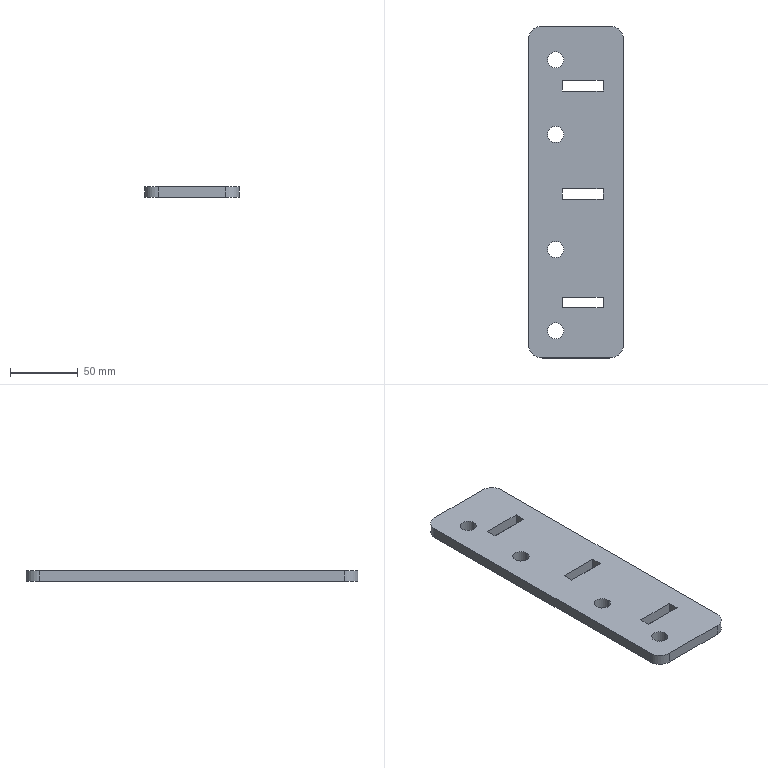Part | SolidWorks | features Fillet 1, FlatPattern 1, SMBaseFlange 1, SheetMetal 1 | 1 solid | 30 faces | box 70 x 245 x 8 mm | volume 127134 mm3 | plane 18 | cylinder 12 | commonest cylinder face diameters 12 x8 20 x4
STEP:
#1=CARTESIAN_POINT('',(-61.919,15.,8.));
#2=VERTEX_POINT('',#1);
#3=CARTESIAN_POINT('',(-49.919,15.,8.));
#4=VERTEX_POINT('',#3);
#5=CARTESIAN_POINT('',(-55.919,15.,8.));
#6=DIRECTION('',(0.,0.,1.));
#7=DIRECTION('',(1.,0.,0.));
#8=AXIS2_PLACEMENT_3D('',#5,#6,#7);
#9=CIRCLE('',#8,6.);
#10=EDGE_CURVE('',#2,#4,#9,.T.);
#11=ORIENTED_EDGE('',*,*,#10,.T.);
#12=CARTESIAN_POINT('',(-49.919,15.,0.));
#13=VERTEX_POINT('',#12);
#14=CARTESIAN_POINT('',(-49.919,15.,8.));
#15=DIRECTION('',(0.,0.,-1.));
#16=VECTOR('',#15,1000.);
#17=LINE('',#14,#16);
#18=EDGE_CURVE('',#4,#13,#17,.T.);
#19=ORIENTED_EDGE('',*,*,#18,.T.);
#20=CARTESIAN_POINT('',(-61.919,15.,0.));
#21=VERTEX_POINT('',#20);
#22=CARTESIAN_POINT('',(-55.919,15.,0.));
#23=DIRECTION('',(0.,0.,1.));
#24=DIRECTION('',(1.,0.,0.));
#25=AXIS2_PLACEMENT_3D('',#22,#23,#24);
#26=CIRCLE('',#25,6.);
#27=EDGE_CURVE('',#21,#13,#26,.T.);
#28=ORIENTED_EDGE('',*,*,#27,.F.);
#29=CARTESIAN_POINT('',(-61.919,15.,8.));
#30=DIRECTION('',(0.,0.,-1.));
#31=VECTOR('',#30,1000.);
#32=LINE('',#29,#31);
#33=EDGE_CURVE('',#2,#21,#32,.T.);
#34=ORIENTED_EDGE('',*,*,#33,.F.);
#35=EDGE_LOOP('',(#11,#19,#28,#34));
#36=FACE_OUTER_BOUND('',#35,.T.);
#37=CARTESIAN_POINT('',(-55.919,15.,8.));
#38=DIRECTION('',(0.,0.,-1.));
#39=DIRECTION('',(-1.,0.,0.));
#40=AXIS2_PLACEMENT_3D('',#37,#38,#39);
#41=CYLINDRICAL_SURFACE('',#40,6.);
#42=ADVANCED_FACE('',(#36),#41,.F.);
#43=CARTESIAN_POINT('',(-61.919,-40.,8.));
#44=VERTEX_POINT('',#43);
#45=CARTESIAN_POINT('',(-49.919,-40.,8.));
#46=VERTEX_POINT('',#45);
#47=CARTESIAN_POINT('',(-55.919,-40.,8.));
#48=DIRECTION('',(0.,0.,1.));
#49=DIRECTION('',(1.,0.,0.));
#50=AXIS2_PLACEMENT_3D('',#47,#48,#49);
#51=CIRCLE('',#50,6.);
#52=EDGE_CURVE('',#44,#46,#51,.T.);
#53=ORIENTED_EDGE('',*,*,#52,.T.);
#54=CARTESIAN_POINT('',(-49.919,-40.,0.));
#55=VERTEX_POINT('',#54);
#56=CARTESIAN_POINT('',(-49.919,-40.,8.));
#57=DIRECTION('',(0.,0.,-1.));
#58=VECTOR('',#57,1000.);
#59=LINE('',#56,#58);
#60=EDGE_CURVE('',#46,#55,#59,.T.);
#61=ORIENTED_EDGE('',*,*,#60,.T.);
#62=CARTESIAN_POINT('',(-61.919,-40.,0.));
#63=VERTEX_POINT('',#62);
#64=CARTESIAN_POINT('',(-55.919,-40.,0.));
#65=DIRECTION('',(0.,0.,1.));
#66=DIRECTION('',(1.,0.,0.));
#67=AXIS2_PLACEMENT_3D('',#64,#65,#66);
#68=CIRCLE('',#67,6.);
#69=EDGE_CURVE('',#63,#55,#68,.T.);
#70=ORIENTED_EDGE('',*,*,#69,.F.);
#71=CARTESIAN_POINT('',(-61.919,-40.,8.));
#72=DIRECTION('',(0.,0.,-1.));
#73=VECTOR('',#72,1000.);
#74=LINE('',#71,#73);
#75=EDGE_CURVE('',#44,#63,#74,.T.);
#76=ORIENTED_EDGE('',*,*,#75,.F.);
#77=EDGE_LOOP('',(#53,#61,#70,#76));
#78=FACE_OUTER_BOUND('',#77,.T.);
#79=CARTESIAN_POINT('',(-55.919,-40.,8.));
#80=DIRECTION('',(0.,0.,-1.));
#81=DIRECTION('',(-1.,0.,0.));
#82=AXIS2_PLACEMENT_3D('',#79,#80,#81);
#83=CYLINDRICAL_SURFACE('',#82,6.);
#84=ADVANCED_FACE('',(#78),#83,.F.);
#85=CARTESIAN_POINT('',(-61.919,-125.,8.));
#86=VERTEX_POINT('',#85);
#87=CARTESIAN_POINT('',(-49.919,-125.,8.));
#88=VERTEX_POINT('',#87);
#89=CARTESIAN_POINT('',(-55.919,-125.,8.));
#90=DIRECTION('',(0.,0.,1.));
#91=DIRECTION('',(1.,0.,0.));
#92=AXIS2_PLACEMENT_3D('',#89,#90,#91);
#93=CIRCLE('',#92,6.);
#94=EDGE_CURVE('',#86,#88,#93,.T.);
#95=ORIENTED_EDGE('',*,*,#94,.T.);
#96=CARTESIAN_POINT('',(-49.919,-125.,0.));
#97=VERTEX_POINT('',#96);
#98=CARTESIAN_POINT('',(-49.919,-125.,8.));
#99=DIRECTION('',(0.,0.,-1.));
#100=VECTOR('',#99,1000.);
#101=LINE('',#98,#100);
#102=EDGE_CURVE('',#88,#97,#101,.T.);
#103=ORIENTED_EDGE('',*,*,#102,.T.);
#104=CARTESIAN_POINT('',(-61.919,-125.,0.));
#105=VERTEX_POINT('',#104);
#106=CARTESIAN_POINT('',(-55.919,-125.,0.));
#107=DIRECTION('',(0.,0.,1.));
#108=DIRECTION('',(1.,0.,0.));
#109=AXIS2_PLACEMENT_3D('',#106,#107,#108);
#110=CIRCLE('',#109,6.);
#111=EDGE_CURVE('',#105,#97,#110,.T.);
#112=ORIENTED_EDGE('',*,*,#111,.F.);
#113=CARTESIAN_POINT('',(-61.919,-125.,8.));
#114=DIRECTION('',(0.,0.,-1.));
#115=VECTOR('',#114,1000.);
#116=LINE('',#113,#115);
#117=EDGE_CURVE('',#86,#105,#116,.T.);
#118=ORIENTED_EDGE('',*,*,#117,.F.);
#119=EDGE_LOOP('',(#95,#103,#112,#118));
#120=FACE_OUTER_BOUND('',#119,.T.);
#121=CARTESIAN_POINT('',(-55.919,-125.,8.));
#122=DIRECTION('',(0.,0.,-1.));
#123=DIRECTION('',(-1.,0.,0.));
#124=AXIS2_PLACEMENT_3D('',#121,#122,#123);
#125=CYLINDRICAL_SURFACE('',#124,6.);
#126=ADVANCED_FACE('',(#120),#125,.F.);
#127=CARTESIAN_POINT('',(-61.919,-185.,8.));
#128=VERTEX_POINT('',#127);
#129=CARTESIAN_POINT('',(-49.919,-185.,8.));
#130=VERTEX_POINT('',#129);
#131=CARTESIAN_POINT('',(-55.919,-185.,8.));
#132=DIRECTION('',(0.,0.,1.));
#133=DIRECTION('',(1.,0.,0.));
#134=AXIS2_PLACEMENT_3D('',#131,#132,#133);
#135=CIRCLE('',#134,6.);
#136=EDGE_CURVE('',#128,#130,#135,.T.);
#137=ORIENTED_EDGE('',*,*,#136,.T.);
#138=CARTESIAN_POINT('',(-49.919,-185.,0.));
#139=VERTEX_POINT('',#138);
#140=CARTESIAN_POINT('',(-49.919,-185.,8.));
#141=DIRECTION('',(0.,0.,-1.));
#142=VECTOR('',#141,1000.);
#143=LINE('',#140,#142);
#144=EDGE_CURVE('',#130,#139,#143,.T.);
#145=ORIENTED_EDGE('',*,*,#144,.T.);
#146=CARTESIAN_POINT('',(-61.919,-185.,0.));
#147=VERTEX_POINT('',#146);
#148=CARTESIAN_POINT('',(-55.919,-185.,0.));
#149=DIRECTION('',(0.,0.,1.));
#150=DIRECTION('',(1.,0.,0.));
#151=AXIS2_PLACEMENT_3D('',#148,#149,#150);
#152=CIRCLE('',#151,6.);
#153=EDGE_CURVE('',#147,#139,#152,.T.);
#154=ORIENTED_EDGE('',*,*,#153,.F.);
#155=CARTESIAN_POINT('',(-61.919,-185.,8.));
#156=DIRECTION('',(0.,0.,-1.));
#157=VECTOR('',#156,1000.);
#158=LINE('',#155,#157);
#159=EDGE_CURVE('',#128,#147,#158,.T.);
#160=ORIENTED_EDGE('',*,*,#159,.F.);
#161=EDGE_LOOP('',(#137,#145,#154,#160));
#162=FACE_OUTER_BOUND('',#161,.T.);
#163=CARTESIAN_POINT('',(-55.919,-185.,8.));
#164=DIRECTION('',(0.,0.,-1.));
#165=DIRECTION('',(-1.,0.,0.));
#166=AXIS2_PLACEMENT_3D('',#163,#164,#165);
#167=CYLINDRICAL_SURFACE('',#166,6.);
#168=ADVANCED_FACE('',(#162),#167,.F.);
#169=ORIENTED_EDGE('',*,*,#52,.F.);
#170=CARTESIAN_POINT('',(-55.919,-40.,8.));
#171=DIRECTION('',(0.,0.,1.));
#172=DIRECTION('',(1.,0.,0.));
#173=AXIS2_PLACEMENT_3D('',#170,#171,#172);
#174=CIRCLE('',#173,6.);
#175=EDGE_CURVE('',#46,#44,#174,.T.);
#176=ORIENTED_EDGE('',*,*,#175,.F.);
#177=EDGE_LOOP('',(#169,#176));
#178=FACE_BOUND('',#177,.T.);
#179=ORIENTED_EDGE('',*,*,#136,.F.);
#180=CARTESIAN_POINT('',(-55.919,-185.,8.));
#181=DIRECTION('',(0.,0.,1.));
#182=DIRECTION('',(1.,0.,0.));
#183=AXIS2_PLACEMENT_3D('',#180,#181,#182);
#184=CIRCLE('',#183,6.);
#185=EDGE_CURVE('',#130,#128,#184,.T.);
#186=ORIENTED_EDGE('',*,*,#185,.F.);
#187=EDGE_LOOP('',(#179,#186));
#188=FACE_BOUND('',#187,.T.);
#189=CARTESIAN_POINT('',(-75.919,30.,8.));
#190=VERTEX_POINT('',#189);
#191=CARTESIAN_POINT('',(-75.919,-195.,8.));
#192=VERTEX_POINT('',#191);
#193=CARTESIAN_POINT('',(-75.919,-205.,8.));
#194=DIRECTION('',(0.,-1.,0.));
#195=VECTOR('',#194,1000.);
#196=LINE('',#193,#195);
#197=EDGE_CURVE('',#190,#192,#196,.T.);
#198=ORIENTED_EDGE('',*,*,#197,.T.);
#199=CARTESIAN_POINT('',(-65.919,-205.,8.));
#200=VERTEX_POINT('',#199);
#201=CARTESIAN_POINT('',(-65.919,-195.,8.));
#202=DIRECTION('',(0.,0.,1.));
#203=DIRECTION('',(1.,0.,0.));
#204=AXIS2_PLACEMENT_3D('',#201,#202,#203);
#205=CIRCLE('',#204,10.);
#206=EDGE_CURVE('',#192,#200,#205,.T.);
#207=ORIENTED_EDGE('',*,*,#206,.T.);
#208=CARTESIAN_POINT('',(-15.919,-205.,8.));
#209=VERTEX_POINT('',#208);
#210=CARTESIAN_POINT('',(-5.919,-205.,8.));
#211=DIRECTION('',(1.,0.,0.));
#212=VECTOR('',#211,1000.);
#213=LINE('',#210,#212);
#214=EDGE_CURVE('',#200,#209,#213,.T.);
#215=ORIENTED_EDGE('',*,*,#214,.T.);
#216=CARTESIAN_POINT('',(-5.919,-195.,8.));
#217=VERTEX_POINT('',#216);
#218=CARTESIAN_POINT('',(-15.919,-195.,8.));
#219=DIRECTION('',(0.,0.,1.));
#220=DIRECTION('',(1.,0.,0.));
#221=AXIS2_PLACEMENT_3D('',#218,#219,#220);
#222=CIRCLE('',#221,10.);
#223=EDGE_CURVE('',#209,#217,#222,.T.);
#224=ORIENTED_EDGE('',*,*,#223,.T.);
#225=CARTESIAN_POINT('',(-5.919,30.,8.));
#226=VERTEX_POINT('',#225);
#227=CARTESIAN_POINT('',(-5.919,-205.,8.));
#228=DIRECTION('',(0.,1.,0.));
#229=VECTOR('',#228,1000.);
#230=LINE('',#227,#229);
#231=EDGE_CURVE('',#217,#226,#230,.T.);
#232=ORIENTED_EDGE('',*,*,#231,.T.);
#233=CARTESIAN_POINT('',(-15.919,40.,8.));
#234=VERTEX_POINT('',#233);
#235=CARTESIAN_POINT('',(-15.919,30.,8.));
#236=DIRECTION('',(0.,0.,1.));
#237=DIRECTION('',(1.,0.,0.));
#238=AXIS2_PLACEMENT_3D('',#235,#236,#237);
#239=CIRCLE('',#238,10.);
#240=EDGE_CURVE('',#226,#234,#239,.T.);
#241=ORIENTED_EDGE('',*,*,#240,.T.);
#242=CARTESIAN_POINT('',(-65.919,40.,8.));
#243=VERTEX_POINT('',#242);
#244=CARTESIAN_POINT('',(-5.919,40.,8.));
#245=DIRECTION('',(-1.,0.,0.));
#246=VECTOR('',#245,1000.);
#247=LINE('',#244,#246);
#248=EDGE_CURVE('',#234,#243,#247,.T.);
#249=ORIENTED_EDGE('',*,*,#248,.T.);
#250=CARTESIAN_POINT('',(-65.919,30.,8.));
#251=DIRECTION('',(0.,0.,1.));
#252=DIRECTION('',(1.,0.,0.));
#253=AXIS2_PLACEMENT_3D('',#250,#251,#252);
#254=CIRCLE('',#253,10.);
#255=EDGE_CURVE('',#243,#190,#254,.T.);
#256=ORIENTED_EDGE('',*,*,#255,.T.);
#257=EDGE_LOOP('',(#198,#207,#215,#224,#232,#241,#249,#256));
#258=FACE_OUTER_BOUND('',#257,.T.);
#259=CARTESIAN_POINT('',(-20.919,-168.,8.));
#260=VERTEX_POINT('',#259);
#261=CARTESIAN_POINT('',(-20.919,-160.,8.));
#262=VERTEX_POINT('',#261);
#263=CARTESIAN_POINT('',(-20.919,-168.,8.));
#264=DIRECTION('',(0.,1.,0.));
#265=VECTOR('',#264,1000.);
#266=LINE('',#263,#265);
#267=EDGE_CURVE('',#260,#262,#266,.T.);
#268=ORIENTED_EDGE('',*,*,#267,.F.);
#269=CARTESIAN_POINT('',(-50.919,-168.,8.));
#270=VERTEX_POINT('',#269);
#271=CARTESIAN_POINT('',(-50.919,-168.,8.));
#272=DIRECTION('',(1.,0.,0.));
#273=VECTOR('',#272,1000.);
#274=LINE('',#271,#273);
#275=EDGE_CURVE('',#270,#260,#274,.T.);
#276=ORIENTED_EDGE('',*,*,#275,.F.);
#277=CARTESIAN_POINT('',(-50.919,-160.,8.));
#278=VERTEX_POINT('',#277);
#279=CARTESIAN_POINT('',(-50.919,-160.,8.));
#280=DIRECTION('',(0.,-1.,0.));
#281=VECTOR('',#280,1000.);
#282=LINE('',#279,#281);
#283=EDGE_CURVE('',#278,#270,#282,.T.);
#284=ORIENTED_EDGE('',*,*,#283,.F.);
#285=CARTESIAN_POINT('',(-20.919,-160.,8.));
#286=DIRECTION('',(-1.,0.,0.));
#287=VECTOR('',#286,1000.);
#288=LINE('',#285,#287);
#289=EDGE_CURVE('',#262,#278,#288,.T.);
#290=ORIENTED_EDGE('',*,*,#289,.F.);
#291=EDGE_LOOP('',(#268,#276,#284,#290));
#292=FACE_BOUND('',#291,.T.);
#293=CARTESIAN_POINT('',(-20.919,-88.,8.));
#294=VERTEX_POINT('',#293);
#295=CARTESIAN_POINT('',(-20.919,-80.,8.));
#296=VERTEX_POINT('',#295);
#297=CARTESIAN_POINT('',(-20.919,-88.,8.));
#298=DIRECTION('',(0.,1.,0.));
#299=VECTOR('',#298,1000.);
#300=LINE('',#297,#299);
#301=EDGE_CURVE('',#294,#296,#300,.T.);
#302=ORIENTED_EDGE('',*,*,#301,.F.);
#303=CARTESIAN_POINT('',(-50.919,-88.,8.));
#304=VERTEX_POINT('',#303);
#305=CARTESIAN_POINT('',(-50.919,-88.,8.));
#306=DIRECTION('',(1.,0.,0.));
#307=VECTOR('',#306,1000.);
#308=LINE('',#305,#307);
#309=EDGE_CURVE('',#304,#294,#308,.T.);
#310=ORIENTED_EDGE('',*,*,#309,.F.);
#311=CARTESIAN_POINT('',(-50.919,-80.,8.));
#312=VERTEX_POINT('',#311);
#313=CARTESIAN_POINT('',(-50.919,-80.,8.));
#314=DIRECTION('',(0.,-1.,0.));
#315=VECTOR('',#314,1000.);
#316=LINE('',#313,#315);
#317=EDGE_CURVE('',#312,#304,#316,.T.);
#318=ORIENTED_EDGE('',*,*,#317,.F.);
#319=CARTESIAN_POINT('',(-20.919,-80.,8.));
#320=DIRECTION('',(-1.,0.,0.));
#321=VECTOR('',#320,1000.);
#322=LINE('',#319,#321);
#323=EDGE_CURVE('',#296,#312,#322,.T.);
#324=ORIENTED_EDGE('',*,*,#323,.F.);
#325=EDGE_LOOP('',(#302,#310,#318,#324));
#326=FACE_BOUND('',#325,.T.);
#327=CARTESIAN_POINT('',(-50.919,-8.,8.));
#328=VERTEX_POINT('',#327);
#329=CARTESIAN_POINT('',(-20.919,-8.,8.));
#330=VERTEX_POINT('',#329);
#331=CARTESIAN_POINT('',(-50.919,-8.,8.));
#332=DIRECTION('',(1.,0.,0.));
#333=VECTOR('',#332,1000.);
#334=LINE('',#331,#333);
#335=EDGE_CURVE('',#328,#330,#334,.T.);
#336=ORIENTED_EDGE('',*,*,#335,.F.);
#337=CARTESIAN_POINT('',(-50.919,0.,8.));
#338=VERTEX_POINT('',#337);
#339=CARTESIAN_POINT('',(-50.919,0.,8.));
#340=DIRECTION('',(0.,-1.,0.));
#341=VECTOR('',#340,1000.);
#342=LINE('',#339,#341);
#343=EDGE_CURVE('',#338,#328,#342,.T.);
#344=ORIENTED_EDGE('',*,*,#343,.F.);
#345=CARTESIAN_POINT('',(-20.919,0.,8.));
#346=VERTEX_POINT('',#345);
#347=CARTESIAN_POINT('',(-20.919,0.,8.));
#348=DIRECTION('',(-1.,0.,0.));
#349=VECTOR('',#348,1000.);
#350=LINE('',#347,#349);
#351=EDGE_CURVE('',#346,#338,#350,.T.);
#352=ORIENTED_EDGE('',*,*,#351,.F.);
#353=CARTESIAN_POINT('',(-20.919,-8.,8.));
#354=DIRECTION('',(0.,1.,0.));
#355=VECTOR('',#354,1000.);
#356=LINE('',#353,#355);
#357=EDGE_CURVE('',#330,#346,#356,.T.);
#358=ORIENTED_EDGE('',*,*,#357,.F.);
#359=EDGE_LOOP('',(#336,#344,#352,#358));
#360=FACE_BOUND('',#359,.T.);
#361=ORIENTED_EDGE('',*,*,#94,.F.);
#362=CARTESIAN_POINT('',(-55.919,-125.,8.));
#363=DIRECTION('',(0.,0.,1.));
#364=DIRECTION('',(1.,0.,0.));
#365=AXIS2_PLACEMENT_3D('',#362,#363,#364);
#366=CIRCLE('',#365,6.);
#367=EDGE_CURVE('',#88,#86,#366,.T.);
#368=ORIENTED_EDGE('',*,*,#367,.F.);
#369=EDGE_LOOP('',(#361,#368));
#370=FACE_BOUND('',#369,.T.);
#371=ORIENTED_EDGE('',*,*,#10,.F.);
#372=CARTESIAN_POINT('',(-55.919,15.,8.));
#373=DIRECTION('',(0.,0.,1.));
#374=DIRECTION('',(1.,0.,0.));
#375=AXIS2_PLACEMENT_3D('',#372,#373,#374);
#376=CIRCLE('',#375,6.);
#377=EDGE_CURVE('',#4,#2,#376,.T.);
#378=ORIENTED_EDGE('',*,*,#377,.F.);
#379=EDGE_LOOP('',(#371,#378));
#380=FACE_BOUND('',#379,.T.);
#381=CARTESIAN_POINT('',(0.,0.,8.));
#382=DIRECTION('',(0.,0.,1.));
#383=DIRECTION('',(1.,0.,0.));
#384=AXIS2_PLACEMENT_3D('',#381,#382,#383);
#385=PLANE('',#384);
#386=ADVANCED_FACE('',(#178,#188,#258,#292,#326,#360,#370,#380),#385,.T.);
#387=CARTESIAN_POINT('',(-50.919,-88.,0.));
#388=VERTEX_POINT('',#387);
#389=CARTESIAN_POINT('',(-20.919,-88.,0.));
#390=VERTEX_POINT('',#389);
#391=CARTESIAN_POINT('',(-50.919,-88.,0.));
#392=DIRECTION('',(1.,0.,0.));
#393=VECTOR('',#392,1000.);
#394=LINE('',#391,#393);
#395=EDGE_CURVE('',#388,#390,#394,.T.);
#396=ORIENTED_EDGE('',*,*,#395,.T.);
#397=CARTESIAN_POINT('',(-20.919,-80.,0.));
#398=VERTEX_POINT('',#397);
#399=CARTESIAN_POINT('',(-20.919,-88.,0.));
#400=DIRECTION('',(0.,1.,0.));
#401=VECTOR('',#400,1000.);
#402=LINE('',#399,#401);
#403=EDGE_CURVE('',#390,#398,#402,.T.);
#404=ORIENTED_EDGE('',*,*,#403,.T.);
#405=CARTESIAN_POINT('',(-50.919,-80.,0.));
#406=VERTEX_POINT('',#405);
#407=CARTESIAN_POINT('',(-20.919,-80.,0.));
#408=DIRECTION('',(-1.,0.,0.));
#409=VECTOR('',#408,1000.);
#410=LINE('',#407,#409);
#411=EDGE_CURVE('',#398,#406,#410,.T.);
#412=ORIENTED_EDGE('',*,*,#411,.T.);
#413=CARTESIAN_POINT('',(-50.919,-80.,0.));
#414=DIRECTION('',(0.,-1.,0.));
#415=VECTOR('',#414,1000.);
#416=LINE('',#413,#415);
#417=EDGE_CURVE('',#406,#388,#416,.T.);
#418=ORIENTED_EDGE('',*,*,#417,.T.);
#419=EDGE_LOOP('',(#396,#404,#412,#418));
#420=FACE_BOUND('',#419,.T.);
#421=CARTESIAN_POINT('',(-65.919,-205.,0.));
#422=VERTEX_POINT('',#421);
#423=CARTESIAN_POINT('',(-15.919,-205.,0.));
#424=VERTEX_POINT('',#423);
#425=CARTESIAN_POINT('',(-5.919,-205.,0.));
#426=DIRECTION('',(1.,0.,0.));
#427=VECTOR('',#426,1000.);
#428=LINE('',#425,#427);
#429=EDGE_CURVE('',#422,#424,#428,.T.);
#430=ORIENTED_EDGE('',*,*,#429,.F.);
#431=CARTESIAN_POINT('',(-75.919,-195.,0.));
#432=VERTEX_POINT('',#431);
#433=CARTESIAN_POINT('',(-65.919,-195.,0.));
#434=DIRECTION('',(0.,0.,-1.));
#435=DIRECTION('',(1.,0.,0.));
#436=AXIS2_PLACEMENT_3D('',#433,#434,#435);
#437=CIRCLE('',#436,10.);
#438=EDGE_CURVE('',#422,#432,#437,.T.);
#439=ORIENTED_EDGE('',*,*,#438,.T.);
#440=CARTESIAN_POINT('',(-75.919,30.,0.));
#441=VERTEX_POINT('',#440);
#442=CARTESIAN_POINT('',(-75.919,-205.,0.));
#443=DIRECTION('',(0.,-1.,0.));
#444=VECTOR('',#443,1000.);
#445=LINE('',#442,#444);
#446=EDGE_CURVE('',#441,#432,#445,.T.);
#447=ORIENTED_EDGE('',*,*,#446,.F.);
#448=CARTESIAN_POINT('',(-65.919,40.,0.));
#449=VERTEX_POINT('',#448);
#450=CARTESIAN_POINT('',(-65.919,30.,0.));
#451=DIRECTION('',(0.,0.,-1.));
#452=DIRECTION('',(1.,0.,0.));
#453=AXIS2_PLACEMENT_3D('',#450,#451,#452);
#454=CIRCLE('',#453,10.);
#455=EDGE_CURVE('',#441,#449,#454,.T.);
#456=ORIENTED_EDGE('',*,*,#455,.T.);
#457=CARTESIAN_POINT('',(-15.919,40.,0.));
#458=VERTEX_POINT('',#457);
#459=CARTESIAN_POINT('',(-5.919,40.,0.));
#460=DIRECTION('',(-1.,0.,0.));
#461=VECTOR('',#460,1000.);
#462=LINE('',#459,#461);
#463=EDGE_CURVE('',#458,#449,#462,.T.);
#464=ORIENTED_EDGE('',*,*,#463,.F.);
#465=CARTESIAN_POINT('',(-5.919,30.,0.));
#466=VERTEX_POINT('',#465);
#467=CARTESIAN_POINT('',(-15.919,30.,0.));
#468=DIRECTION('',(0.,0.,-1.));
#469=DIRECTION('',(1.,0.,0.));
#470=AXIS2_PLACEMENT_3D('',#467,#468,#469);
#471=CIRCLE('',#470,10.);
#472=EDGE_CURVE('',#458,#466,#471,.T.);
#473=ORIENTED_EDGE('',*,*,#472,.T.);
#474=CARTESIAN_POINT('',(-5.919,-195.,0.));
#475=VERTEX_POINT('',#474);
#476=CARTESIAN_POINT('',(-5.919,-205.,0.));
#477=DIRECTION('',(0.,1.,0.));
#478=VECTOR('',#477,1000.);
#479=LINE('',#476,#478);
#480=EDGE_CURVE('',#475,#466,#479,.T.);
#481=ORIENTED_EDGE('',*,*,#480,.F.);
#482=CARTESIAN_POINT('',(-15.919,-195.,0.));
#483=DIRECTION('',(0.,0.,-1.));
#484=DIRECTION('',(1.,0.,0.));
#485=AXIS2_PLACEMENT_3D('',#482,#483,#484);
#486=CIRCLE('',#485,10.);
#487=EDGE_CURVE('',#475,#424,#486,.T.);
#488=ORIENTED_EDGE('',*,*,#487,.T.);
#489=EDGE_LOOP('',(#430,#439,#447,#456,#464,#473,#481,#488));
#490=FACE_OUTER_BOUND('',#489,.T.);
#491=CARTESIAN_POINT('',(-50.919,-168.,0.));
#492=VERTEX_POINT('',#491);
#493=CARTESIAN_POINT('',(-20.919,-168.,0.));
#494=VERTEX_POINT('',#493);
#495=CARTESIAN_POINT('',(-50.919,-168.,0.));
#496=DIRECTION('',(1.,0.,0.));
#497=VECTOR('',#496,1000.);
#498=LINE('',#495,#497);
#499=EDGE_CURVE('',#492,#494,#498,.T.);
#500=ORIENTED_EDGE('',*,*,#499,.T.);
#501=CARTESIAN_POINT('',(-20.919,-160.,0.));
#502=VERTEX_POINT('',#501);
#503=CARTESIAN_POINT('',(-20.919,-168.,0.));
#504=DIRECTION('',(0.,1.,0.));
#505=VECTOR('',#504,1000.);
#506=LINE('',#503,#505);
#507=EDGE_CURVE('',#494,#502,#506,.T.);
#508=ORIENTED_EDGE('',*,*,#507,.T.);
#509=CARTESIAN_POINT('',(-50.919,-160.,0.));
#510=VERTEX_POINT('',#509);
#511=CARTESIAN_POINT('',(-20.919,-160.,0.));
#512=DIRECTION('',(-1.,0.,0.));
#513=VECTOR('',#512,1000.);
#514=LINE('',#511,#513);
#515=EDGE_CURVE('',#502,#510,#514,.T.);
#516=ORIENTED_EDGE('',*,*,#515,.T.);
#517=CARTESIAN_POINT('',(-50.919,-160.,0.));
#518=DIRECTION('',(0.,-1.,0.));
#519=VECTOR('',#518,1000.);
#520=LINE('',#517,#519);
#521=EDGE_CURVE('',#510,#492,#520,.T.);
#522=ORIENTED_EDGE('',*,*,#521,.T.);
#523=EDGE_LOOP('',(#500,#508,#516,#522));
#524=FACE_BOUND('',#523,.T.);
#525=CARTESIAN_POINT('',(-50.919,0.,0.));
#526=VERTEX_POINT('',#525);
#527=CARTESIAN_POINT('',(-50.919,-8.,0.));
#528=VERTEX_POINT('',#527);
#529=CARTESIAN_POINT('',(-50.919,0.,0.));
#530=DIRECTION('',(0.,-1.,0.));
#531=VECTOR('',#530,1000.);
#532=LINE('',#529,#531);
#533=EDGE_CURVE('',#526,#528,#532,.T.);
#534=ORIENTED_EDGE('',*,*,#533,.T.);
#535=CARTESIAN_POINT('',(-20.919,-8.,0.));
#536=VERTEX_POINT('',#535);
#537=CARTESIAN_POINT('',(-50.919,-8.,0.));
#538=DIRECTION('',(1.,0.,0.));
#539=VECTOR('',#538,1000.);
#540=LINE('',#537,#539);
#541=EDGE_CURVE('',#528,#536,#540,.T.);
#542=ORIENTED_EDGE('',*,*,#541,.T.);
#543=CARTESIAN_POINT('',(-20.919,0.,0.));
#544=VERTEX_POINT('',#543);
#545=CARTESIAN_POINT('',(-20.919,-8.,0.));
#546=DIRECTION('',(0.,1.,0.));
#547=VECTOR('',#546,1000.);
#548=LINE('',#545,#547);
#549=EDGE_CURVE('',#536,#544,#548,.T.);
#550=ORIENTED_EDGE('',*,*,#549,.T.);
#551=CARTESIAN_POINT('',(-20.919,0.,0.));
#552=DIRECTION('',(-1.,0.,0.));
#553=VECTOR('',#552,1000.);
#554=LINE('',#551,#553);
#555=EDGE_CURVE('',#544,#526,#554,.T.);
#556=ORIENTED_EDGE('',*,*,#555,.T.);
#557=EDGE_LOOP('',(#534,#542,#550,#556));
#558=FACE_BOUND('',#557,.T.);
#559=ORIENTED_EDGE('',*,*,#153,.T.);
#560=CARTESIAN_POINT('',(-55.919,-185.,0.));
#561=DIRECTION('',(0.,0.,1.));
#562=DIRECTION('',(1.,0.,0.));
#563=AXIS2_PLACEMENT_3D('',#560,#561,#562);
#564=CIRCLE('',#563,6.);
#565=EDGE_CURVE('',#139,#147,#564,.T.);
#566=ORIENTED_EDGE('',*,*,#565,.T.);
#567=EDGE_LOOP('',(#559,#566));
#568=FACE_BOUND('',#567,.T.);
#569=ORIENTED_EDGE('',*,*,#111,.T.);
#570=CARTESIAN_POINT('',(-55.919,-125.,0.));
#571=DIRECTION('',(0.,0.,1.));
#572=DIRECTION('',(1.,0.,0.));
#573=AXIS2_PLACEMENT_3D('',#570,#571,#572);
#574=CIRCLE('',#573,6.);
#575=EDGE_CURVE('',#97,#105,#574,.T.);
#576=ORIENTED_EDGE('',*,*,#575,.T.);
#577=EDGE_LOOP('',(#569,#576));
#578=FACE_BOUND('',#577,.T.);
#579=ORIENTED_EDGE('',*,*,#69,.T.);
#580=CARTESIAN_POINT('',(-55.919,-40.,0.));
#581=DIRECTION('',(0.,0.,1.));
#582=DIRECTION('',(1.,0.,0.));
#583=AXIS2_PLACEMENT_3D('',#580,#581,#582);
#584=CIRCLE('',#583,6.);
#585=EDGE_CURVE('',#55,#63,#584,.T.);
#586=ORIENTED_EDGE('',*,*,#585,.T.);
#587=EDGE_LOOP('',(#579,#586));
#588=FACE_BOUND('',#587,.T.);
#589=ORIENTED_EDGE('',*,*,#27,.T.);
#590=CARTESIAN_POINT('',(-55.919,15.,0.));
#591=DIRECTION('',(0.,0.,1.));
#592=DIRECTION('',(1.,0.,0.));
#593=AXIS2_PLACEMENT_3D('',#590,#591,#592);
#594=CIRCLE('',#593,6.);
#595=EDGE_CURVE('',#13,#21,#594,.T.);
#596=ORIENTED_EDGE('',*,*,#595,.T.);
#597=EDGE_LOOP('',(#589,#596));
#598=FACE_BOUND('',#597,.T.);
#599=CARTESIAN_POINT('',(0.,0.,0.));
#600=DIRECTION('',(0.,0.,1.));
#601=DIRECTION('',(1.,0.,0.));
#602=AXIS2_PLACEMENT_3D('',#599,#600,#601);
#603=PLANE('',#602);
#604=ADVANCED_FACE('',(#420,#490,#524,#558,#568,#578,#588,#598),#603,.F.);
#605=ORIENTED_EDGE('',*,*,#231,.F.);
#606=CARTESIAN_POINT('',(-5.919,-195.,8.));
#607=DIRECTION('',(0.,0.,-1.));
#608=VECTOR('',#607,1000.);
#609=LINE('',#606,#608);
#610=EDGE_CURVE('',#217,#475,#609,.T.);
#611=ORIENTED_EDGE('',*,*,#610,.T.);
#612=ORIENTED_EDGE('',*,*,#480,.T.);
#613=CARTESIAN_POINT('',(-5.919,30.,8.));
#614=DIRECTION('',(0.,0.,1.));
#615=VECTOR('',#614,1000.);
#616=LINE('',#613,#615);
#617=EDGE_CURVE('',#466,#226,#616,.T.);
#618=ORIENTED_EDGE('',*,*,#617,.T.);
#619=EDGE_LOOP('',(#605,#611,#612,#618));
#620=FACE_OUTER_BOUND('',#619,.T.);
#621=CARTESIAN_POINT('',(-5.919,-205.,8.));
#622=DIRECTION('',(-1.,0.,0.));
#623=DIRECTION('',(0.,-1.,0.));
#624=AXIS2_PLACEMENT_3D('',#621,#622,#623);
#625=PLANE('',#624);
#626=ADVANCED_FACE('',(#620),#625,.F.);
#627=ORIENTED_EDGE('',*,*,#248,.F.);
#628=CARTESIAN_POINT('',(-15.919,40.,8.));
#629=DIRECTION('',(0.,0.,-1.));
#630=VECTOR('',#629,1000.);
#631=LINE('',#628,#630);
#632=EDGE_CURVE('',#234,#458,#631,.T.);
#633=ORIENTED_EDGE('',*,*,#632,.T.);
#634=ORIENTED_EDGE('',*,*,#463,.T.);
#635=CARTESIAN_POINT('',(-65.919,40.,8.));
#636=DIRECTION('',(0.,0.,1.));
#637=VECTOR('',#636,1000.);
#638=LINE('',#635,#637);
#639=EDGE_CURVE('',#449,#243,#638,.T.);
#640=ORIENTED_EDGE('',*,*,#639,.T.);
#641=EDGE_LOOP('',(#627,#633,#634,#640));
#642=FACE_OUTER_BOUND('',#641,.T.);
#643=CARTESIAN_POINT('',(-5.919,40.,8.));
#644=DIRECTION('',(0.,-1.,0.));
#645=DIRECTION('',(1.,0.,0.));
#646=AXIS2_PLACEMENT_3D('',#643,#644,#645);
#647=PLANE('',#646);
#648=ADVANCED_FACE('',(#642),#647,.F.);
#649=ORIENTED_EDGE('',*,*,#446,.T.);
#650=CARTESIAN_POINT('',(-75.919,-195.,8.));
#651=DIRECTION('',(0.,0.,1.));
#652=VECTOR('',#651,1000.);
#653=LINE('',#650,#652);
#654=EDGE_CURVE('',#432,#192,#653,.T.);
#655=ORIENTED_EDGE('',*,*,#654,.T.);
#656=ORIENTED_EDGE('',*,*,#197,.F.);
#657=CARTESIAN_POINT('',(-75.919,30.,8.));
#658=DIRECTION('',(0.,0.,-1.));
#659=VECTOR('',#658,1000.);
#660=LINE('',#657,#659);
#661=EDGE_CURVE('',#190,#441,#660,.T.);
#662=ORIENTED_EDGE('',*,*,#661,.T.);
#663=EDGE_LOOP('',(#649,#655,#656,#662));
#664=FACE_OUTER_BOUND('',#663,.T.);
#665=CARTESIAN_POINT('',(-75.919,-205.,8.));
#666=DIRECTION('',(1.,0.,0.));
#667=DIRECTION('',(0.,0.,-1.));
#668=AXIS2_PLACEMENT_3D('',#665,#666,#667);
#669=PLANE('',#668);
#670=ADVANCED_FACE('',(#664),#669,.F.);
#671=ORIENTED_EDGE('',*,*,#214,.F.);
#672=CARTESIAN_POINT('',(-65.919,-205.,8.));
#673=DIRECTION('',(0.,0.,-1.));
#674=VECTOR('',#673,1000.);
#675=LINE('',#672,#674);
#676=EDGE_CURVE('',#200,#422,#675,.T.);
#677=ORIENTED_EDGE('',*,*,#676,.T.);
#678=ORIENTED_EDGE('',*,*,#429,.T.);
#679=CARTESIAN_POINT('',(-15.919,-205.,8.));
#680=DIRECTION('',(0.,0.,1.));
#681=VECTOR('',#680,1000.);
#682=LINE('',#679,#681);
#683=EDGE_CURVE('',#424,#209,#682,.T.);
#684=ORIENTED_EDGE('',*,*,#683,.T.);
#685=EDGE_LOOP('',(#671,#677,#678,#684));
#686=FACE_OUTER_BOUND('',#685,.T.);
#687=CARTESIAN_POINT('',(-5.919,-205.,8.));
#688=DIRECTION('',(0.,1.,0.));
#689=DIRECTION('',(0.,0.,1.));
#690=AXIS2_PLACEMENT_3D('',#687,#688,#689);
#691=PLANE('',#690);
#692=ADVANCED_FACE('',(#686),#691,.F.);
#693=ORIENTED_EDGE('',*,*,#499,.F.);
#694=CARTESIAN_POINT('',(-50.919,-168.,8.));
#695=DIRECTION('',(0.,0.,-1.));
#696=VECTOR('',#695,1000.);
#697=LINE('',#694,#696);
#698=EDGE_CURVE('',#270,#492,#697,.T.);
#699=ORIENTED_EDGE('',*,*,#698,.F.);
#700=ORIENTED_EDGE('',*,*,#275,.T.);
#701=CARTESIAN_POINT('',(-20.919,-168.,8.));
#702=DIRECTION('',(0.,0.,-1.));
#703=VECTOR('',#702,1000.);
#704=LINE('',#701,#703);
#705=EDGE_CURVE('',#260,#494,#704,.T.);
#706=ORIENTED_EDGE('',*,*,#705,.T.);
#707=EDGE_LOOP('',(#693,#699,#700,#706));
#708=FACE_OUTER_BOUND('',#707,.T.);
#709=CARTESIAN_POINT('',(-50.919,-168.,8.));
#710=DIRECTION('',(0.,1.,0.));
#711=DIRECTION('',(0.,0.,1.));
#712=AXIS2_PLACEMENT_3D('',#709,#710,#711);
#713=PLANE('',#712);
#714=ADVANCED_FACE('',(#708),#713,.T.);
#715=ORIENTED_EDGE('',*,*,#507,.F.);
#716=ORIENTED_EDGE('',*,*,#705,.F.);
#717=ORIENTED_EDGE('',*,*,#267,.T.);
#718=CARTESIAN_POINT('',(-20.919,-160.,8.));
#719=DIRECTION('',(0.,0.,-1.));
#720=VECTOR('',#719,1000.);
#721=LINE('',#718,#720);
#722=EDGE_CURVE('',#262,#502,#721,.T.);
#723=ORIENTED_EDGE('',*,*,#722,.T.);
#724=EDGE_LOOP('',(#715,#716,#717,#723));
#725=FACE_OUTER_BOUND('',#724,.T.);
#726=CARTESIAN_POINT('',(-20.919,-168.,8.));
#727=DIRECTION('',(-1.,0.,0.));
#728=DIRECTION('',(0.,0.,1.));
#729=AXIS2_PLACEMENT_3D('',#726,#727,#728);
#730=PLANE('',#729);
#731=ADVANCED_FACE('',(#725),#730,.T.);
#732=ORIENTED_EDGE('',*,*,#515,.F.);
#733=ORIENTED_EDGE('',*,*,#722,.F.);
#734=ORIENTED_EDGE('',*,*,#289,.T.);
#735=CARTESIAN_POINT('',(-50.919,-160.,8.));
#736=DIRECTION('',(0.,0.,-1.));
#737=VECTOR('',#736,1000.);
#738=LINE('',#735,#737);
#739=EDGE_CURVE('',#278,#510,#738,.T.);
#740=ORIENTED_EDGE('',*,*,#739,.T.);
#741=EDGE_LOOP('',(#732,#733,#734,#740));
#742=FACE_OUTER_BOUND('',#741,.T.);
#743=CARTESIAN_POINT('',(-20.919,-160.,8.));
#744=DIRECTION('',(0.,-1.,0.));
#745=DIRECTION('',(0.,0.,-1.));
#746=AXIS2_PLACEMENT_3D('',#743,#744,#745);
#747=PLANE('',#746);
#748=ADVANCED_FACE('',(#742),#747,.T.);
#749=ORIENTED_EDGE('',*,*,#521,.F.);
#750=ORIENTED_EDGE('',*,*,#739,.F.);
#751=ORIENTED_EDGE('',*,*,#283,.T.);
#752=ORIENTED_EDGE('',*,*,#698,.T.);
#753=EDGE_LOOP('',(#749,#750,#751,#752));
#754=FACE_OUTER_BOUND('',#753,.T.);
#755=CARTESIAN_POINT('',(-50.919,-160.,8.));
#756=DIRECTION('',(1.,0.,0.));
#757=DIRECTION('',(0.,0.,-1.));
#758=AXIS2_PLACEMENT_3D('',#755,#756,#757);
#759=PLANE('',#758);
#760=ADVANCED_FACE('',(#754),#759,.T.);
#761=ORIENTED_EDGE('',*,*,#395,.F.);
#762=CARTESIAN_POINT('',(-50.919,-88.,8.));
#763=DIRECTION('',(0.,0.,-1.));
#764=VECTOR('',#763,1000.);
#765=LINE('',#762,#764);
#766=EDGE_CURVE('',#304,#388,#765,.T.);
#767=ORIENTED_EDGE('',*,*,#766,.F.);
#768=ORIENTED_EDGE('',*,*,#309,.T.);
#769=CARTESIAN_POINT('',(-20.919,-88.,8.));
#770=DIRECTION('',(0.,0.,-1.));
#771=VECTOR('',#770,1000.);
#772=LINE('',#769,#771);
#773=EDGE_CURVE('',#294,#390,#772,.T.);
#774=ORIENTED_EDGE('',*,*,#773,.T.);
#775=EDGE_LOOP('',(#761,#767,#768,#774));
#776=FACE_OUTER_BOUND('',#775,.T.);
#777=CARTESIAN_POINT('',(-50.919,-88.,8.));
#778=DIRECTION('',(0.,1.,0.));
#779=DIRECTION('',(0.,0.,1.));
#780=AXIS2_PLACEMENT_3D('',#777,#778,#779);
#781=PLANE('',#780);
#782=ADVANCED_FACE('',(#776),#781,.T.);
#783=ORIENTED_EDGE('',*,*,#403,.F.);
#784=ORIENTED_EDGE('',*,*,#773,.F.);
#785=ORIENTED_EDGE('',*,*,#301,.T.);
#786=CARTESIAN_POINT('',(-20.919,-80.,8.));
#787=DIRECTION('',(0.,0.,-1.));
#788=VECTOR('',#787,1000.);
#789=LINE('',#786,#788);
#790=EDGE_CURVE('',#296,#398,#789,.T.);
#791=ORIENTED_EDGE('',*,*,#790,.T.);
#792=EDGE_LOOP('',(#783,#784,#785,#791));
#793=FACE_OUTER_BOUND('',#792,.T.);
#794=CARTESIAN_POINT('',(-20.919,-88.,8.));
#795=DIRECTION('',(-1.,0.,0.));
#796=DIRECTION('',(0.,0.,1.));
#797=AXIS2_PLACEMENT_3D('',#794,#795,#796);
#798=PLANE('',#797);
#799=ADVANCED_FACE('',(#793),#798,.T.);
#800=ORIENTED_EDGE('',*,*,#411,.F.);
#801=ORIENTED_EDGE('',*,*,#790,.F.);
#802=ORIENTED_EDGE('',*,*,#323,.T.);
#803=CARTESIAN_POINT('',(-50.919,-80.,8.));
#804=DIRECTION('',(0.,0.,-1.));
#805=VECTOR('',#804,1000.);
#806=LINE('',#803,#805);
#807=EDGE_CURVE('',#312,#406,#806,.T.);
#808=ORIENTED_EDGE('',*,*,#807,.T.);
#809=EDGE_LOOP('',(#800,#801,#802,#808));
#810=FACE_OUTER_BOUND('',#809,.T.);
#811=CARTESIAN_POINT('',(-20.919,-80.,8.));
#812=DIRECTION('',(0.,-1.,0.));
#813=DIRECTION('',(0.,0.,-1.));
#814=AXIS2_PLACEMENT_3D('',#811,#812,#813);
#815=PLANE('',#814);
#816=ADVANCED_FACE('',(#810),#815,.T.);
#817=ORIENTED_EDGE('',*,*,#417,.F.);
#818=ORIENTED_EDGE('',*,*,#807,.F.);
#819=ORIENTED_EDGE('',*,*,#317,.T.);
#820=ORIENTED_EDGE('',*,*,#766,.T.);
#821=EDGE_LOOP('',(#817,#818,#819,#820));
#822=FACE_OUTER_BOUND('',#821,.T.);
#823=CARTESIAN_POINT('',(-50.919,-80.,8.));
#824=DIRECTION('',(1.,0.,0.));
#825=DIRECTION('',(0.,0.,-1.));
#826=AXIS2_PLACEMENT_3D('',#823,#824,#825);
#827=PLANE('',#826);
#828=ADVANCED_FACE('',(#822),#827,.T.);
#829=ORIENTED_EDGE('',*,*,#533,.F.);
#830=CARTESIAN_POINT('',(-50.919,0.,8.));
#831=DIRECTION('',(0.,0.,-1.));
#832=VECTOR('',#831,1000.);
#833=LINE('',#830,#832);
#834=EDGE_CURVE('',#338,#526,#833,.T.);
#835=ORIENTED_EDGE('',*,*,#834,.F.);
#836=ORIENTED_EDGE('',*,*,#343,.T.);
#837=CARTESIAN_POINT('',(-50.919,-8.,8.));
#838=DIRECTION('',(0.,0.,-1.));
#839=VECTOR('',#838,1000.);
#840=LINE('',#837,#839);
#841=EDGE_CURVE('',#328,#528,#840,.T.);
#842=ORIENTED_EDGE('',*,*,#841,.T.);
#843=EDGE_LOOP('',(#829,#835,#836,#842));
#844=FACE_OUTER_BOUND('',#843,.T.);
#845=CARTESIAN_POINT('',(-50.919,0.,8.));
#846=DIRECTION('',(1.,0.,0.));
#847=DIRECTION('',(0.,0.,-1.));
#848=AXIS2_PLACEMENT_3D('',#845,#846,#847);
#849=PLANE('',#848);
#850=ADVANCED_FACE('',(#844),#849,.T.);
#851=ORIENTED_EDGE('',*,*,#541,.F.);
#852=ORIENTED_EDGE('',*,*,#841,.F.);
#853=ORIENTED_EDGE('',*,*,#335,.T.);
#854=CARTESIAN_POINT('',(-20.919,-8.,8.));
#855=DIRECTION('',(0.,0.,-1.));
#856=VECTOR('',#855,1000.);
#857=LINE('',#854,#856);
#858=EDGE_CURVE('',#330,#536,#857,.T.);
#859=ORIENTED_EDGE('',*,*,#858,.T.);
#860=EDGE_LOOP('',(#851,#852,#853,#859));
#861=FACE_OUTER_BOUND('',#860,.T.);
#862=CARTESIAN_POINT('',(-50.919,-8.,8.));
#863=DIRECTION('',(0.,1.,0.));
#864=DIRECTION('',(0.,0.,1.));
#865=AXIS2_PLACEMENT_3D('',#862,#863,#864);
#866=PLANE('',#865);
#867=ADVANCED_FACE('',(#861),#866,.T.);
#868=ORIENTED_EDGE('',*,*,#549,.F.);
#869=ORIENTED_EDGE('',*,*,#858,.F.);
#870=ORIENTED_EDGE('',*,*,#357,.T.);
#871=CARTESIAN_POINT('',(-20.919,0.,8.));
#872=DIRECTION('',(0.,0.,-1.));
#873=VECTOR('',#872,1000.);
#874=LINE('',#871,#873);
#875=EDGE_CURVE('',#346,#544,#874,.T.);
#876=ORIENTED_EDGE('',*,*,#875,.T.);
#877=EDGE_LOOP('',(#868,#869,#870,#876));
#878=FACE_OUTER_BOUND('',#877,.T.);
#879=CARTESIAN_POINT('',(-20.919,-8.,8.));
#880=DIRECTION('',(-1.,0.,0.));
#881=DIRECTION('',(0.,0.,1.));
#882=AXIS2_PLACEMENT_3D('',#879,#880,#881);
#883=PLANE('',#882);
#884=ADVANCED_FACE('',(#878),#883,.T.);
#885=ORIENTED_EDGE('',*,*,#555,.F.);
#886=ORIENTED_EDGE('',*,*,#875,.F.);
#887=ORIENTED_EDGE('',*,*,#351,.T.);
#888=ORIENTED_EDGE('',*,*,#834,.T.);
#889=EDGE_LOOP('',(#885,#886,#887,#888));
#890=FACE_OUTER_BOUND('',#889,.T.);
#891=CARTESIAN_POINT('',(-20.919,0.,8.));
#892=DIRECTION('',(0.,-1.,0.));
#893=DIRECTION('',(1.,0.,0.));
#894=AXIS2_PLACEMENT_3D('',#891,#892,#893);
#895=PLANE('',#894);
#896=ADVANCED_FACE('',(#890),#895,.T.);
#897=ORIENTED_EDGE('',*,*,#144,.F.);
#898=ORIENTED_EDGE('',*,*,#185,.T.);
#899=ORIENTED_EDGE('',*,*,#159,.T.);
#900=ORIENTED_EDGE('',*,*,#565,.F.);
#901=EDGE_LOOP('',(#897,#898,#899,#900));
#902=FACE_OUTER_BOUND('',#901,.T.);
#903=CARTESIAN_POINT('',(-55.919,-185.,8.));
#904=DIRECTION('',(0.,0.,-1.));
#905=DIRECTION('',(-1.,0.,0.));
#906=AXIS2_PLACEMENT_3D('',#903,#904,#905);
#907=CYLINDRICAL_SURFACE('',#906,6.);
#908=ADVANCED_FACE('',(#902),#907,.F.);
#909=ORIENTED_EDGE('',*,*,#102,.F.);
#910=ORIENTED_EDGE('',*,*,#367,.T.);
#911=ORIENTED_EDGE('',*,*,#117,.T.);
#912=ORIENTED_EDGE('',*,*,#575,.F.);
#913=EDGE_LOOP('',(#909,#910,#911,#912));
#914=FACE_OUTER_BOUND('',#913,.T.);
#915=CARTESIAN_POINT('',(-55.919,-125.,8.));
#916=DIRECTION('',(0.,0.,-1.));
#917=DIRECTION('',(-1.,0.,0.));
#918=AXIS2_PLACEMENT_3D('',#915,#916,#917);
#919=CYLINDRICAL_SURFACE('',#918,6.);
#920=ADVANCED_FACE('',(#914),#919,.F.);
#921=ORIENTED_EDGE('',*,*,#60,.F.);
#922=ORIENTED_EDGE('',*,*,#175,.T.);
#923=ORIENTED_EDGE('',*,*,#75,.T.);
#924=ORIENTED_EDGE('',*,*,#585,.F.);
#925=EDGE_LOOP('',(#921,#922,#923,#924));
#926=FACE_OUTER_BOUND('',#925,.T.);
#927=CARTESIAN_POINT('',(-55.919,-40.,8.));
#928=DIRECTION('',(0.,0.,-1.));
#929=DIRECTION('',(-1.,0.,0.));
#930=AXIS2_PLACEMENT_3D('',#927,#928,#929);
#931=CYLINDRICAL_SURFACE('',#930,6.);
#932=ADVANCED_FACE('',(#926),#931,.F.);
#933=ORIENTED_EDGE('',*,*,#18,.F.);
#934=ORIENTED_EDGE('',*,*,#377,.T.);
#935=ORIENTED_EDGE('',*,*,#33,.T.);
#936=ORIENTED_EDGE('',*,*,#595,.F.);
#937=EDGE_LOOP('',(#933,#934,#935,#936));
#938=FACE_OUTER_BOUND('',#937,.T.);
#939=CARTESIAN_POINT('',(-55.919,15.,8.));
#940=DIRECTION('',(0.,0.,-1.));
#941=DIRECTION('',(-1.,0.,0.));
#942=AXIS2_PLACEMENT_3D('',#939,#940,#941);
#943=CYLINDRICAL_SURFACE('',#942,6.);
#944=ADVANCED_FACE('',(#938),#943,.F.);
#945=ORIENTED_EDGE('',*,*,#206,.F.);
#946=ORIENTED_EDGE('',*,*,#654,.F.);
#947=ORIENTED_EDGE('',*,*,#438,.F.);
#948=ORIENTED_EDGE('',*,*,#676,.F.);
#949=EDGE_LOOP('',(#945,#946,#947,#948));
#950=FACE_OUTER_BOUND('',#949,.T.);
#951=CARTESIAN_POINT('',(-65.919,-195.,8.));
#952=DIRECTION('',(0.,0.,-1.));
#953=DIRECTION('',(-1.,0.,0.));
#954=AXIS2_PLACEMENT_3D('',#951,#952,#953);
#955=CYLINDRICAL_SURFACE('',#954,10.);
#956=ADVANCED_FACE('',(#950),#955,.T.);
#957=ORIENTED_EDGE('',*,*,#223,.F.);
#958=ORIENTED_EDGE('',*,*,#683,.F.);
#959=ORIENTED_EDGE('',*,*,#487,.F.);
#960=ORIENTED_EDGE('',*,*,#610,.F.);
#961=EDGE_LOOP('',(#957,#958,#959,#960));
#962=FACE_OUTER_BOUND('',#961,.T.);
#963=CARTESIAN_POINT('',(-15.919,-195.,8.));
#964=DIRECTION('',(0.,0.,-1.));
#965=DIRECTION('',(-1.,0.,0.));
#966=AXIS2_PLACEMENT_3D('',#963,#964,#965);
#967=CYLINDRICAL_SURFACE('',#966,10.);
#968=ADVANCED_FACE('',(#962),#967,.T.);
#969=ORIENTED_EDGE('',*,*,#240,.F.);
#970=ORIENTED_EDGE('',*,*,#617,.F.);
#971=ORIENTED_EDGE('',*,*,#472,.F.);
#972=ORIENTED_EDGE('',*,*,#632,.F.);
#973=EDGE_LOOP('',(#969,#970,#971,#972));
#974=FACE_OUTER_BOUND('',#973,.T.);
#975=CARTESIAN_POINT('',(-15.919,30.,8.));
#976=DIRECTION('',(0.,0.,-1.));
#977=DIRECTION('',(-1.,0.,0.));
#978=AXIS2_PLACEMENT_3D('',#975,#976,#977);
#979=CYLINDRICAL_SURFACE('',#978,10.);
#980=ADVANCED_FACE('',(#974),#979,.T.);
#981=ORIENTED_EDGE('',*,*,#255,.F.);
#982=ORIENTED_EDGE('',*,*,#639,.F.);
#983=ORIENTED_EDGE('',*,*,#455,.F.);
#984=ORIENTED_EDGE('',*,*,#661,.F.);
#985=EDGE_LOOP('',(#981,#982,#983,#984));
#986=FACE_OUTER_BOUND('',#985,.T.);
#987=CARTESIAN_POINT('',(-65.919,30.,8.));
#988=DIRECTION('',(0.,0.,-1.));
#989=DIRECTION('',(-1.,0.,0.));
#990=AXIS2_PLACEMENT_3D('',#987,#988,#989);
#991=CYLINDRICAL_SURFACE('',#990,10.);
#992=ADVANCED_FACE('',(#986),#991,.T.);
#993=CLOSED_SHELL('',(#42,#84,#126,#168,#386,#604,#626,#648,#670,#692,#714,#731,#748,#760,#782,#799,#816,#828,#850,#867,#884,#896,#908,#920,#932,#944,#956,#968,#980,#992));
#994=MANIFOLD_SOLID_BREP('',#993);
#995=CARTESIAN_POINT('',(0.,0.,0.));
#996=DIRECTION('',(0.,0.,1.));
#997=DIRECTION('',(1.,0.,0.));
#998=AXIS2_PLACEMENT_3D('',#995,#996,#997);
#999=(LENGTH_UNIT()NAMED_UNIT(*)SI_UNIT(.MILLI.,.METRE.));
#1000=UNCERTAINTY_MEASURE_WITH_UNIT(LENGTH_MEASURE(0.00001),#999,'','');
#1001=(NAMED_UNIT(*)PLANE_ANGLE_UNIT()SI_UNIT($,.RADIAN.));
#1002=(NAMED_UNIT(*)SI_UNIT($,.STERADIAN.)SOLID_ANGLE_UNIT());
#1003=(GEOMETRIC_REPRESENTATION_CONTEXT(3)GLOBAL_UNCERTAINTY_ASSIGNED_CONTEXT((#1000))GLOBAL_UNIT_ASSIGNED_CONTEXT((#999,#1001,#1002))REPRESENTATION_CONTEXT('',''));
#1004=ADVANCED_BREP_SHAPE_REPRESENTATION('',(#994,#998),#1003);